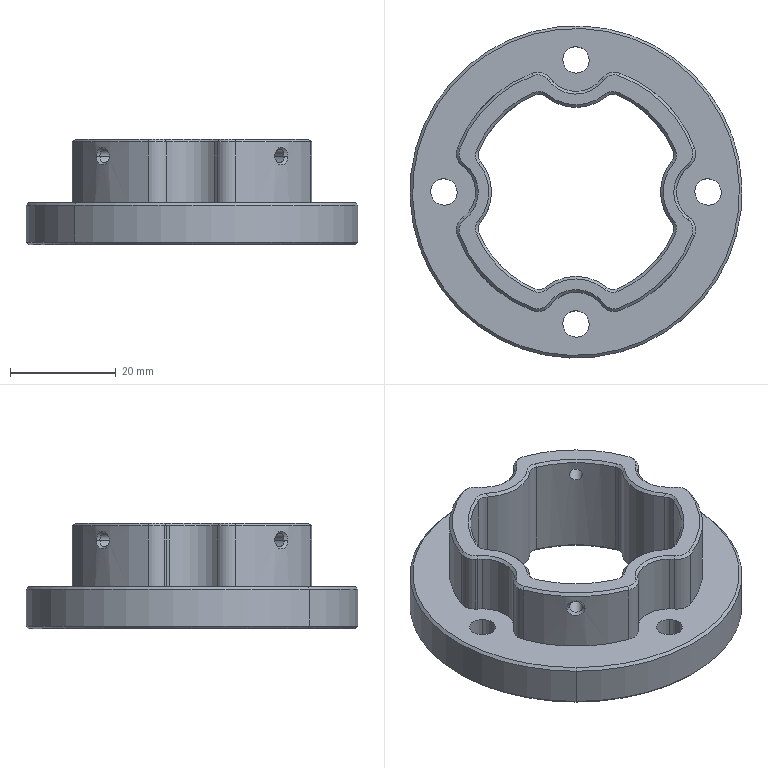NC program | NX | posted with a generic post | part box 62.9 x 62.9 x 20 mm
Lines 19 to 903 of 7695:
(ADAPTIVE_MILLING , TOOL : D10)
N36 T15 M6
N38 G54
N40 G17 G0 G90 X-44.154 Y6.39 S9500 M3
N42 G43 Z30. H15
N44 Z-8.9
N46 G94 G1 Z-11.9 F1000.
N48 X-43.177 Y6.446 F3000.
N50 X-42.201 Y6.527
N52 G3 X-41.498 Y7.102 R1.025
N54 X-40.854 Y10.262 R9.424
N56 X-40.658 Y21.758 R185.073
N58 G2 X-40.625 Y34.257 R639.071
N60 X-37.724 Y38.491 R6.067
N62 X-32.153 Y40.276 R13.146
N64 X-22.865 Y40.627 R85.364
N66 G1 X-21.065 Y40.633
N68 X-18.265 Y40.637
N70 X-12.065 Y40.639
N72 X33.735
N74 X33.835 Y40.637
N76 X33.935 Y40.634
N78 G2 X38.31 Y37.975 R5.843
N80 X40.247 Y32.358 R12.556
N82 X40.625 Y23.371 R77.114
N84 G1 X40.631 Y21.771
N86 X40.635 Y19.571
N88 X40.638 Y15.471
N90 X40.639 Y-15.229
N92 Y-33.729
N94 X40.638 Y-33.829
N96 G2 X37.978 Y-38.306 R5.815
N98 X32.461 Y-40.233 R12.425
N100 X24.476 Y-40.617 R66.82
N102 G1 X23.276 Y-40.625
N104 X21.676 Y-40.631
N106 X19.376 Y-40.636
N108 X15.076 Y-40.638
N110 X-33.724 Y-40.639
N112 X-33.824 Y-40.638
N114 G2 X-38.303 Y-37.982 R5.813
N116 X-40.22 Y-32.565 R12.366
N118 X-40.617 Y-24.481 R65.384
N120 G1 X-40.625 Y-23.381
N122 X-40.631 Y-21.781
N124 X-40.636 Y-19.481
N126 X-40.638 Y-15.281
N128 X-40.639 Y3.719
N130 X-40.637 Y3.919
N132 G2 X-40.169 Y9.298 R115.764
N134 G3 X-39.871 Y21.891 R175.546
N136 G1 X-39.867 Y24.891
N138 X-39.865 Y30.991
N140 X-39.863 Y31.091
N142 X-39.861 Y31.191
N144 X-39.853 Y31.391
N146 X-39.847 Y31.491
N148 X-39.84 Y31.59
N150 G2 X-36.002 Y37.476 R7.669
N152 X-29.749 Y39.423 R15.539
N154 X-19.762 Y39.816 R92.027
N156 G1 X-18.062 Y39.822
N158 X-15.662 Y39.827
N160 X-11.462 Y39.829
N162 X11.738 Y39.83
N164 X30.938
N166 X31.138 Y39.829
N168 G2 X37.449 Y36.019 R7.595
N170 X39.403 Y29.871 R15.313
N172 X39.808 Y20.986 R79.126
N174 G1 X39.816 Y19.686
N176 X39.822 Y17.986
N178 X39.827 Y15.486
N180 X39.829 Y11.186
N182 X39.83 Y-16.914
N184 Y-30.914
N186 G2 X36.123 Y-37.383 R7.547
N188 X29.795 Y-39.414 R15.249
N190 X20.609 Y-39.811 R83.586
N192 G1 X19.209 Y-39.818
N194 X17.309 Y-39.824
N196 X14.409 Y-39.828
N198 X8.509 Y-39.83
N200 X-30.991
N202 X-31.091
N204 G2 X-37.425 Y-36.057 R7.589
N206 X-39.413 Y-29.818 R15.258
N208 X-39.81 Y-20.632 R83.029
N210 G1 X-39.818 Y-19.132
N212 X-39.824 Y-17.232
N214 X-39.828 Y-14.332
N216 X-39.83 Y-8.332
N218 Y1.668
N220 X-39.827 Y2.068
N222 G2 X-39.346 Y9.852 R183.612
N224 G3 X-39.076 Y27.048 R323.967
N226 G2 X-38.811 Y31.028 R16.814
N228 X-33.821 Y36.948 R9.086
N230 X-26.878 Y38.692 R19.542
N232 X-15.986 Y39.011 R133.202
N234 G1 X-13.786 Y39.016
N236 X-10.386 Y39.02
N238 X-2.386 Y39.021
N240 X28.614
N242 X28.814 Y39.02
N244 X29.014 Y39.016
N246 G2 X36.75 Y34.168 R8.812
N248 X38.616 Y27.57 R18.024
N250 X39.001 Y18.082 R95.38
N252 G1 X39.009 Y16.582
N254 X39.015 Y14.582
N256 X39.019 Y11.682
N258 X39.021 Y5.982
N260 Y-28.618
N262 X39.02 Y-28.818
N264 G2 X34.163 Y-36.752 R8.824
N266 X27.365 Y-38.636 R18.17
N268 X16.675 Y-39.007 R112.972
N270 G1 X14.875 Y-39.014
N272 X12.276 Y-39.018
N274 X7.576 Y-39.021
N276 X-26.124 Y-39.022
N278 X-28.624 Y-39.021
N280 X-28.924 Y-39.018
N282 G2 X-36.708 Y-34.246 R8.797
N284 X-38.627 Y-27.459 R17.966
N286 X-39.008 Y-16.471 R114.033
N288 G1 X-39.014 Y-14.571
N290 X-39.019 Y-11.771
N292 X-39.021 Y-6.571
N294 Y0.029
N296 X-39.018 Y0.529
N298 X-39.012 Y1.029
N300 G2 X-38.485 Y11.415 R472.51
N302 G3 X-38.266 Y27.212 R522.18
N304 G2 X-32.726 Y35.942 R9.729
N306 X-25.911 Y37.789 R19.648
N308 X-14.624 Y38.197 R113.317
N310 G1 X-12.724 Y38.204
N312 X-10.124 Y38.209
N314 X-5.724 Y38.212
N316 X10.776 Y38.213
N318 X26.476
N320 X26.776 Y38.211
N322 G2 X36.02 Y32.533 R9.762
N324 X37.86 Y25.203 R20.771
N326 X38.204 Y12.812 R149.811
N328 G1 X38.209 Y10.212
N330 X38.212 Y5.812
N332 X38.213 Y-10.688
N334 Y-26.488
N336 X38.211 Y-26.788
N338 X38.207 Y-26.988
N340 G2 X32.609 Y-35.98 R9.723
N342 X25.686 Y-37.808 R19.975
N344 X14.497 Y-38.198 R118.542
N346 G1 X12.597 Y-38.204
N348 X9.997 Y-38.209
N350 X5.497 Y-38.212
N352 X-12.803 Y-38.213
N354 X-26.503
N356 X-26.803 Y-38.211
N358 G2 X-35.987 Y-32.599 R9.746
N360 X-37.832 Y-25.476 R20.283
N362 X-38.201 Y-13.686 R131.503
N364 X-38.158 Y1.813 R695.009
N366 G3 X-37.586 Y15.301 R684.53
N368 G2 X-37.441 Y26.099 R805.731
N370 X-31.332 Y35.151 R10.389
N372 X-24.004 Y37.007 R21.646
N374 X-13.314 Y37.384 R121.368
N376 G1 X-11.614 Y37.392
N378 X-9.314 Y37.398
N380 X-6.014 Y37.402
N382 X0.686 Y37.404
N384 X24.686
N386 X24.886 Y37.403
N388 G2 X30.856 Y36.034 R11.659
N390 X35.671 Y30.094 R11.361
N392 X37.144 Y22.363 R26.659
N394 X37.4 Y7.967 R242.401
N396 G1 X37.403 Y3.567
N398 X37.404 Y-11.633
N400 Y-24.633
N402 X37.403 Y-24.833
N404 X37.397 Y-25.232
N406 X37.393 Y-25.432
N408 G2 X34.427 Y-32.947 R10.423
N410 X27.757 Y-36.386 R13.873
N412 X19.32 Y-37.29 R43.09
N414 X2.72 Y-37.403 R760.11
N416 G1 X-18.28 Y-37.404
N418 X-24.68
N420 X-24.979 Y-37.402
N422 X-25.379 Y-37.395
N424 X-25.579 Y-37.39
N426 X-25.779 Y-37.382
N428 G2 X-35.059 Y-31.472 R10.331
N430 X-37.006 Y-23.965 R21.227
N432 X-37.39 Y-12.175 R132.868
N434 X-37.295 Y2.723 R384.936
N436 G3 X-36.678 Y24.012 R473.575
N438 G2 X-34.552 Y30.768 R11.574
N440 X-28.011 Y35.141 R12.771
N442 X-19.929 Y36.39 R32.975
N444 X-3.032 Y36.594 R394.511
N446 G1 X5.668 Y36.596
N448 X22.868
N450 X23.468 Y36.59
N452 X23.768 Y36.585
N454 X24.068 Y36.577
N456 G2 X31.057 Y34.264 R11.324
N458 X35.223 Y27.696 R13.034
N460 X36.406 Y19.501 R34.517
N462 X36.594 Y2.504 R426.496
N464 G1 X36.596 Y-7.396
N466 Y-22.896
N468 X36.59 Y-23.496
N470 X36.587 Y-23.696
N472 X36.576 Y-24.096
N474 G2 X34.118 Y-31.232 R11.22
N476 X27.475 Y-35.287 R13.274
N478 X19.371 Y-36.413 R35.677
N480 X5.273 Y-36.592 R366.726
N482 G1 X0.173 Y-36.595
N484 X-22.827 Y-36.596
N486 X-23.127 Y-36.595
N488 X-23.527 Y-36.589
N490 X-23.927 Y-36.581
N492 X-24.126 Y-36.574
N494 G2 X-31.332 Y-34.036 R11.175
N496 X-35.323 Y-27.351 R13.41
N498 X-36.427 Y-19.043 R36.843
N500 X-36.171 Y10.047 R355.609
N502 G3 X-35.886 Y22.644 R750.66
N504 G2 X-33.985 Y29.285 R12.572
N506 X-27.318 Y34.141 R12.741
N508 X-19.162 Y35.537 R31.275
N510 X-4.366 Y35.782 R280.79
N512 G1 X0.034 Y35.786
N514 X12.034 Y35.787
N516 X21.234
N518 X21.834 Y35.781
N520 X22.234 Y35.775
N522 X22.434 Y35.77
N524 G2 X28.859 Y34.17 R12.771
N526 X33.942 Y27.81 R12.264
N528 X35.481 Y19.886 R28.128
N530 X35.78 Y5.592 R220.124
N532 G1 X35.785 Y2.192
N534 X35.787 Y-4.408
N536 Y-21.308
N538 X35.785 Y-21.708
N540 X35.779 Y-22.108
N542 X35.77 Y-22.508
N544 G2 X34.026 Y-29.093 R12.572
N546 X27.456 Y-34.07 R12.532
N548 X19.411 Y-35.514 R29.843
N550 X4.516 Y-35.782 R258.634
N552 G1 X0.316 Y-35.786
N554 X-10.084 Y-35.787
N556 X-21.284
N558 X-21.884 Y-35.781
N560 X-22.184 Y-35.777
N562 X-22.584 Y-35.766
N564 G2 X-29.326 Y-33.879 R12.376
N566 X-34.163 Y-27.198 R12.759
N568 X-35.523 Y-19.338 R31.138
N570 X-35.778 Y-3.042 R287.727
N572 X-35.261 Y13.849 R960.15
N574 X-35.022 Y22.444 R183.444
N576 X-27.881 Y32.632 R11.828
N578 X-19.948 Y34.554 R24.698
N580 X-8.459 Y34.955 R134.916
N582 G1 X-6.959 Y34.963
N584 X-4.959 Y34.97
N586 X-2.059 Y34.974
N588 X2.841 Y34.978
N590 X19.641 Y34.979
N592 X20.141 Y34.976
N594 G2 X26.05 Y34.14 R17.215
N596 X32.764 Y27.517 R11.889
N598 X34.566 Y19.757 R25.348
N600 X34.961 Y7.367 R147.215
N602 G1 X34.969 Y5.267
N604 X34.974 Y2.467
N606 X34.977 Y-2.033
N608 X34.979 Y-14.333
N610 X34.978 Y-19.833
N612 X34.977 Y-20.133
N614 G2 X34.213 Y-25.854 R17.552
N616 X27.705 Y-32.677 R11.823
N618 X20.063 Y-34.535 R24.423
N620 X7.375 Y-34.961 R140.259
N622 G1 X5.275 Y-34.969
N624 X2.375 Y-34.974
N626 X-2.225 Y-34.977
N628 X-15.225 Y-34.979
N630 X-19.725 Y-34.978
N632 X-20.125 Y-34.976
N634 G2 X-26.036 Y-34.148 R17.243
N636 X-32.634 Y-27.807 R11.793
N638 X-34.564 Y-19.775 R24.739
N640 X-34.962 Y-7.185 R150.047
N642 X-34.53 Y11.708 R466.509
N644 X-34.245 Y21.103 R252.318
N646 X-30.784 Y29.092 R12.363
N648 X-23.638 Y32.911 R15.397
N650 X-14.321 Y34.016 R44.534
N652 X9.177 Y34.17 R850.322
N654 X20.776 Y34.105 R348.279
N656 X28.27 Y31.428 R12.545
N658 X32.61 Y24.608 R14.088
N660 X33.922 Y16.231 R35.311
N662 X34.166 Y0.035 R327.22
N664 G1 X34.169 Y-4.765
N666 X34.17 Y-18.265
N668 X34.168 Y-18.765
N670 X34.16 Y-19.265
N672 X34.152 Y-19.665
N674 G2 X32.838 Y-26.077 R15.03
N676 X26.124 Y-32.062 R12.55
N678 X18.039 Y-33.791 R27.574
N680 X6.048 Y-34.151 R158.399
N682 G1 X3.948 Y-34.159
N684 X1.548 Y-34.164
N686 X-2.552 Y-34.168
N688 X-11.652 Y-34.17
N690 X-18.252
N692 X-18.852 Y-34.165
N694 G2 X-24.867 Y-33.347 R18.267
N696 X-31.777 Y-26.78 R12.083
N698 X-33.717 Y-18.851 R24.92
N700 X-34.145 Y-7.064 R133.048
N702 X-33.746 Y11.531 R521.596
N704 X-33.439 Y20.124 R169.021
N706 X-29.523 Y28.531 R12.614
N708 X-22.072 Y32.204 R16.367
N710 X-12.741 Y33.216 R49.308
N712 X10.657 Y33.361 R912.675
N714 X20.055 Y33.258 R166.649
N716 X28.363 Y29.591 R12.423
N718 X32.101 Y22.397 R15.794
N720 X33.204 Y12.978 R46.108
N722 X33.36 Y-5.82 R649.081
N724 X33.308 Y-19.319 R520.164
N726 X31.273 Y-26.338 R13.629
N728 X24.439 Y-31.473 R13.459
N730 X16.112 Y-33.037 R31.178
N732 X2.618 Y-33.35 R213.351
N734 G1 X-0.082 Y-33.355
N736 X-4.082 Y-33.359
N738 X-12.682 Y-33.361
N740 X-16.882
N742 X-17.482 Y-33.356
N744 X-18.082 Y-33.347
N746 G2 X-24.266 Y-32.348 R17.235
N748 X-30.97 Y-25.68 R12.456
N750 X-32.914 Y-17.547 R25.856
N752 X-33.316 Y-2.758 R151.885
N754 X-33.089 Y6.739 R611.107
N756 X-32.703 Y18.432 R406.653
N758 X-30.307 Y25.748 R14.076
N760 X-23.14 Y30.775 R14.212
N762 X-14.591 Y32.25 R33.829
N764 X1.604 Y32.547 R280.622
N766 X18.003 Y32.502 R718.96
N768 X24.987 Y30.664 R14.521
N770 X30.579 Y23.584 R13.493
N772 X32.203 Y15.168 R30.977
N774 X32.543 Y0.375 R220.032
N776 X32.503 Y-18.025 R842.566
N778 X30.551 Y-25.177 R14.375
N780 X23.659 Y-30.551 R13.569
N782 X15.347 Y-32.19 R30.306
N784 X1.255 Y-32.541 R202.046
N786 G1 X-1.445 Y-32.547
N788 X-5.545 Y-32.551
N790 X-14.045 Y-32.553
N792 X-15.645 Y-32.552
N794 X-16.245 Y-32.549
N796 X-16.745 Y-32.541
N798 G2 X-22.949 Y-31.632 R18.901
N800 X-30.098 Y-24.75 R12.628
N802 X-32.106 Y-16.326 R26.295
N804 X-32.487 Y-1.637 R144.765
N806 X-31.935 Y17.154 R631.236
N808 X-29.939 Y24.1 R15.089
N810 X-22.755 Y29.729 R13.907
N812 X-14.342 Y31.371 R31.231
N814 X-1.149 Y31.727 R191.229
N816 X16.55 Y31.702 R884.582
N818 X23.33 Y30.205 R15.959
N820 X29.526 Y23.148 R13.281
N822 X31.338 Y14.673 R29.244
N824 X31.729 Y0.582 R186.623
N826 X31.695 Y-16.818 R780.638
N828 X30.036 Y-23.655 R15.347
N830 X22.995 Y-29.591 R13.469
N832 X14.707 Y-31.336 R29.368
N834 X0.916 Y-31.728 R180.86
N836 X-16.883 Y-31.691 R726.882
N838 X-23.799 Y-29.957 R15.111
N840 X-29.578 Y-23.029 R13.489
N842 X-31.362 Y-14.445 R29.894
N844 X-31.601 Y1.746 R164.804
N846 X-31.147 Y16.138 R407.692
N848 X-29.054 Y23.26 R15.315
N850 X-21.852 Y28.874 R14.108
N852 X-13.144 Y30.568 R31.918
N854 X1.648 Y30.924 R222.232
N856 X15.648 Y30.882 R578.884
N858 X22.596 Y29.251 R15.856
N860 X28.64 Y22.303 R13.463
N862 X30.501 Y13.839 R29.013
N864 X30.914 Y0.749 R163.434
N866 X30.886 Y-15.65 R709.93
N868 X29.252 Y-22.598 R15.884
N870 X22.118 Y-28.719 R13.567
N872 X13.639 Y-30.521 R29.782
N874 X0.949 Y-30.912 R168.52
N876 X-15.75 Y-30.881 R618.315
N878 X-22.599 Y-29.255 R15.737
N880 X-28.682 Y-22.213 R13.552
N882 X-30.503 Y-13.841 R29.011
N884 X-30.793 Y1.249 R143.854
N886 X-30.368 Y15.041 R354.424
N888 X-28.327 Y22.185 R15.914
N890 X-21.128 Y27.958 R14.207
N892 X-12.536 Y29.716 R31.047
N894 X1.055 Y30.107 R179.958
N896 X14.754 Y30.063 R430.554
N898 X21.784 Y28.352 R15.989
N900 X27.875 Y21.185 R13.8
N902 X29.691 Y12.708 R29.863
N904 X30.111 Y-1.881 R184.764
N906 X30.054 Y-14.98 R357.073
N908 X28.144 Y-22.155 R15.422
N910 X20.978 Y-27.963 R14.017
N912 X12.486 Y-29.713 R30.736
N914 X-1.705 Y-30.11 R189.354
N916 X-14.904 Y-30.057 R375.136
N918 X-21.914 Y-28.279 R15.627
N920 X-27.784 Y-21.42 R13.724
N922 X-29.7 Y-12.663 R29.361
N924 X-29.953 Y2.528 R147.815
N926 X-29.567 Y14.22 R242.398
N928 X-27.354 Y21.514 R15.754
N930 X-19.967 Y27.214 R14.541
N932 X-11.262 Y28.926 R32.658
N934 X2.23 Y29.298 R193.523
N936 X13.829 Y29.245 R301.238
N938 X20.857 Y27.52 R16.145
N940 X27.102 Y20.104 R14.055
N942 X28.88 Y11.618 R30.801
N944 X29.295 Y-1.672 R168.302
N946 X29.235 Y-14.071 R290.213
N948 X27.353 Y-21.155 R15.684
N950 X19.975 Y-27.155 R14.144
N952 X11.38 Y-28.905 R31.529
N954 X-2.01 Y-29.297 R182.206
N956 X-13.909 Y-29.24 R308.785
N958 X-21.014 Y-27.43 R15.897
N960 X-27.061 Y-20.217 R14.025
N962 X-28.911 Y-11.24 R30.857
N964 X-29.121 Y3.253 R150.199
N966 X-28.748 Y13.544 R166.987
N968 X-26.19 Y21.129 R15.346
N970 X-18.583 Y26.553 R15.107
N972 X-9.652 Y28.158 R35.45
N974 X6.242 Y28.499 R259.089
N976 X14.236 Y28.325 R86.731
N978 X22.699 Y24.672 R13.839
N980 X26.966 Y17.096 R16.45
N982 X28.278 Y7.505 R43.892
N984 X28.435 Y-12.791 R341.832
N986 X26.653 Y-20.008 R16.436
N988 X19.325 Y-26.214 R14.125
N990 X10.752 Y-28.054 R30.216
N992 X-3.538 Y-28.49 R180.341
N994 X-13.435 Y-28.393 R166.547
N996 X-20.986 Y-26.054 R15.058
N998 X-26.414 Y-18.814 R14.653
N1000 X-28.115 Y-9.905 R32.989
N1002 X-28.297 Y3.589 R145.776
N1004 X-27.939 Y12.78 R127.958
N1006 X-25.241 Y20.418 R15.291
N1008 X-17.759 Y25.696 R15.302
N1010 X-10.069 Y27.247 R35.598
N1012 X-7.887 Y27.73 R9.388
N1014 G3 X6.761 Y27.73 R374.985
N1016 G2 X14.247 Y27.388 R56.312
N1018 X25.007 Y19.273 R13.607
N1020 X27.115 Y10.973 R27.235
N1022 G3 X27.269 Y10.003 R6.674
N1024 G2 X27.728 Y6.561 R9.435
N1026 G3 X27.72 Y-8.786 R480.733
N1028 G2 X27.146 Y-15.549 R33.036
N1030 X19.617 Y-24.848 R13.474
N1032 X11.35 Y-27.07 R26.12
N1034 G3 X8.415 Y-27.667 R14.624
N1036 G2 X3.962 Y-27.67 R54.526
N1038 X-10.26 Y-27.687 R749.013
N1040 X-16.873 Y-26.777 R22.801
N1042 X-25.011 Y-19.276 R13.604
N1044 X-27.136 Y-10.674 R27.209
N1046 G3 X-27.516 Y-9.201 R6.554
N1048 G2 X-27.689 Y-6.116 R10.038
N1050 G3 X-27.474 Y5.18 R696.749
N1052 G2 X-27.569 Y9.108 R9.238
N1054 X-26.546 Y15.215 R37.091
N1056 X-18.57 Y24.184 R14.105
N1058 X-13.236 Y25.851 R25.594
N1060 G1 X-10.069 Y27.247
N1062 G2 X-7.887 Y27.73 R8.71
N1064 G1 X-6.219 Y27.687
N1066 G3 X-0.369 Y26.961 R22.412
N1068 G1 X0.23 Y26.947
N1070 X0.93 Y26.935
N1072 X1.73 Y26.926
N1074 X2.73 Y26.918
N1076 X3.53 Y26.915
N1078 X3.63 Y26.922
N1080 X3.729 Y26.937
N1082 G2 X6.547 Y27.72 R9.23
N1084 G3 X6.343 Y29.901 R1.1
N1086 G1 X4.344 Y29.834 Z-11.8
N1088 X-3.496 Y29.566
N1090 X-4.145 Y29.549 Z-11.833
N1092 X-4.793 Y29.508 Z-11.865
N1094 G3 X-5.394 Y29.171 Z-11.9 R1.144
N1096 X-4.845 Y27.361 R1.102
N1098 G2 X-3.497 Y26.854 R12.893
N1100 G3 X2.449 Y26.247 R20.794
N1102 X3.37 Y26.765 R3.244
N1104 G1 X3.923 Y26.998
N1106 G3 X4.401 Y28.637 R1.103
N1108 X3.408 Y29.113 Z-11.843 R1.131
N1110 G1 X2.559 Y29.117 Z-11.8
N1112 X-2.62 Y29.147
N1114 X-3.18 Y29.154 Z-11.828
N1116 X-3.741 Y29.139 Z-11.856
N1118 G3 X-4.469 Y28.689 Z-11.9 R1.128
N1120 X-4.058 Y27.066 R1.103
N1122 X1.627 Y25.68 R10.558
N1124 X2.819 Y26.392 R3.71
N1126 X2.224 Y28.391 R1.101
N1128 G1 X-2.324 Y28.549
N1130 G3 X-2.952 Y26.521 R1.101
N1132 X1.156 Y25.238 R5.804
N1134 X1.945 Y25.777 R1.631
N1136 G1 X2.026 Y25.834
N1138 G3 X1.507 Y27.828 R1.101
N1140 G1 X-1.745 Y28.165
N1142 G3 X-2.544 Y26.211 R1.101
N1144 X0.386 Y24.853 R4.842
N1146 X1.698 Y25.526 R1.473
N1148 X1.016 Y27.362 R1.101
N1150 G1 X-1.027 Y27.602
N1152 G3 X-1.841 Y25.65 R1.101
N1154 X-0.598 Y24.766 R4.738
N1156 X1.025 Y24.814 R1.654
N1158 G1 X1.102 Y24.878
N1160 X1.373 Y25.172
N1162 G3 X0.715 Y27.006 R1.101
N1164 G1 X0.011 Y27.11
N1166 X-0.697 Y27.189
N1168 G3 X-1.505 Y25.37 R1.101
N1170 X0.344 Y24.385 R2.116
N1172 X1.11 Y24.886 R1.337
N1174 X0.436 Y26.722 R1.101
N1176 G1 X0.026 Y26.774
N1178 X-0.386 Y26.81
N1180 G3 X-1.179 Y24.992 R1.101
N1182 X0.144 Y24.233 R1.554
N1184 X0.932 Y24.692 R1.248
N1186 X-1.144 Y25.935 R-1.233
N1188 X-0.917 Y24.689 R1.261
N1190 X0.712 Y24.469 R1.083
N1192 G1 X0.797 Y24.545
N1194 X1.86 Y25.703
N1196 X1.945 Y25.777
N1198 G2 X4.973 Y27.427 R9.279
N1200 G1 X6.661 Y27.733
N1202 X6.761 Y27.73
N1204 G2 X9.871 Y27.307 R9.014
N1206 X14.975 Y26.325 R72.636
N1208 X24.226 Y18.271 R13.984
N1210 X25.819 Y13.273 R29.214
N1212 X27.242 Y10.083 R41.896
N1214 G3 X28.775 Y9.69 R1.003
N1216 X29.176 Y10.531 Z-11.852 R1.137
N1218 G1 X29.316 Y11.559 Z-11.8
N1220 X29.455 Y12.566
N1222 X29.579 Y13.575
N1224 X29.553 Y13.781
N1226 X29.492 Y13.98
N1228 X27.962 Y17.399
N1230 X26.396 Y20.802
N1232 G3 X25.029 Y22.866 R9.239
N1234 G1 X23.629 Y24.461
N1236 X22.211 Y26.038
N1238 G3 X19.802 Y27.776 R9.636
N1240 G1 X19.128 Y28.101
N1242 X18.44 Y28.392
N1244 X12.857 Y30.533
N1246 G3 X12.056 Y30.495 R1.026
N1248 G1 X10.524 Y29.737
N1250 X9.923 Y29.445 Z-11.833
N1252 X9.333 Y29.131 Z-11.867
N1254 G3 X8.958 Y28.599 Z-11.9 R1.04
N1256 X9.676 Y27.351 R1.004
N1258 G2 X11.558 Y26.623 R15.109
N1260 X16.247 Y24.898 R43.642
N1262 X23.698 Y16.731 R15.105
N1264 X25.823 Y13.266 R25.695
N1266 G3 X27.669 Y13.539 R1.001
N1268 X27.633 Y14.204 Z-11.867 R1.689
N1270 G1 X27.414 Y15.515 Z-11.8
N1272 X27.096 Y17.375
N1274 X26.988 Y17.613
N1276 X25.636 Y19.785
N1278 X24.27 Y21.947
N1280 G3 X22.073 Y24.696 R21.386
N1282 X19.539 Y26.601 R10.917
N1284 G1 X15.082 Y29.016
N1286 G3 X14.457 Y29.126 R1.042
N1288 G1 X12.673 Y28.859
N1290 X11.979 Y28.758 Z-11.835
N1292 X11.287 Y28.641 Z-11.87
N1294 G3 X10.801 Y28.311 Z-11.9 R1.049
N1296 X11.184 Y26.766 R1.003
N1298 G1 X12.908 Y26.023
N1300 X12.959 Y25.998
N1302 G2 X17.491 Y23.171 R33.094
N1304 X20.588 Y20.493 R35.872
N1306 G1 X22.637 Y18.204
N1308 X22.672 Y18.16
N1310 X23.722 Y16.698
N1312 G3 X25.38 Y18.13 R-1.1
N1314 G1 X17.103 Y26.126
N1316 G3 X15.696 Y24.443 R-1.1
N1318 G1 X17.806 Y22.923
N1320 G2 X20.588 Y20.493 R35.704
N1322 X24.494 Y15.616 R33.992
N1324 G1 X26.031 Y12.891
N1326 X27.269 Y10.003
N1328 G2 X27.733 Y6.661 R9.461
N1330 G3 X27.063 Y2.403 R37.637
N1332 X26.934 Y-3.694 R104.126
N1334 G1 X27.346 Y-4.71
N1336 X27.687 Y-6.21
N1338 X27.7 Y-6.316
N1340 G3 X29.854 Y-6.465 R1.1
N1342 G1 X29.892 Y-6.111 Z-11.882
N1344 X29.88 Y-5.756 Z-11.864
N1346 X29.843 Y-4.469 Z-11.8
N1348 X29.609 Y3.686
N1350 X29.595 Y4.27 Z-11.829
N1352 X29.563 Y4.854 Z-11.859
N1354 G3 X29.135 Y5.542 Z-11.9 R1.13
N1356 X27.427 Y4.973 R1.102
N1358 X26.334 Y0.319 R12.438
N1360 X26.258 Y-2.476 R18.046
N1362 X26.676 Y-3.209 R2.933
N1364 G1 X27.007 Y-3.937
N1366 G3 X28.622 Y-4.395 R1.103
N1368 X29.108 Y-3.299 Z-11.837 R1.19
N1370 G1 X29.11 Y-2.559 Z-11.8
N1372 X29.119 Y2.501
N1374 X29.123 Y3.09 Z-11.829
N1376 X29.109 Y3.679 Z-11.859
N1378 G3 X28.71 Y4.375 Z-11.9 R1.13
N1380 X27.007 Y3.944 R1.103
N1382 G1 X26.765 Y3.37
N1384 X26.711 Y3.272
N1386 X26.656 Y3.188
N1388 X26.604 Y3.103
N1390 X26.556 Y3.015
N1392 X26.509 Y2.927
N1394 X26.465 Y2.837
N1396 X26.423 Y2.746
N1398 X26.383 Y2.655
N1400 X26.344 Y2.563
N1402 X26.308 Y2.47
N1404 X26.273 Y2.376
N1406 G3 X25.688 Y-1.655 R10.536
N1408 X26.42 Y-2.84 R3.647
N1410 X28.407 Y-2.26 R1.101
N1412 G1 X28.708 Y2.57
N1414 G3 X26.711 Y3.272 R1.101
N1416 X25.225 Y-1.072 R6.432
N1418 X25.716 Y-1.874 R1.396
N1420 G1 X25.833 Y-2.035
N1422 G3 X27.817 Y-1.494 R1.101
N1424 G1 X28.13 Y1.714
N1426 G3 X26.136 Y2.454 R1.101
N1428 X25.046 Y0.634 R6.657
N1430 X24.997 Y-1.123 R2.397
N1432 X25.543 Y-1.702 R3.429
N1434 X27.378 Y-0.981 R1.101
N1436 G1 X27.543 Y0.957
N1438 G3 X25.703 Y1.86 R1.101
N1440 X24.633 Y-0.677 R2.61
N1442 X25.181 Y-1.374 R1.696
N1444 X27.012 Y-0.695 R1.101
N1446 G1 X27.108 Y0.028
N1448 X27.178 Y0.754
N1450 G3 X25.335 Y1.522 R1.101
N1452 X24.384 Y-0.35 R2.169
N1454 X24.888 Y-1.107 R1.341
N1456 X26.719 Y-0.429 R1.101
N1458 G1 X26.772 Y-0.008
N1460 X26.81 Y0.416
N1462 G3 X24.966 Y1.184 R1.101
N1464 X24.231 Y-0.154 R1.583
N1466 X24.696 Y-0.933 R1.257
N1468 X26.41 Y0.691 R1.185
N1470 X24.598 Y0.846 R1.238
N1472 X24.468 Y-0.709 R1.071
N1474 G1 X24.548 Y-0.799
N1476 X25.139 Y-1.328
N1478 X25.716 Y-1.874
N1480 X26.205 Y-2.534
N1482 X26.676 Y-3.209
N1484 X27.021 Y-3.955
N1486 X27.346 Y-4.71
N1488 X27.534 Y-5.511
N1490 X27.7 Y-6.316
N1492 X27.73 Y-7.886
N1494 G2 X27.186 Y-10.617 R28.474
N1496 X25.952 Y-16.173 R31.711
N1498 X18.043 Y-24.332 R14.053
N1500 X13.278 Y-25.816 R28.776
N1502 X10.083 Y-27.242 R42.262
N1504 G3 X9.69 Y-28.775 R1.003
N1506 X10.531 Y-29.176 Z-11.852 R1.137
N1508 G1 X11.559 Y-29.316 Z-11.8
N1510 X12.566 Y-29.455
N1512 X13.575 Y-29.579
N1514 X13.781 Y-29.553
N1516 X13.98 Y-29.492
N1518 X17.399 Y-27.962
N1520 X20.802 Y-26.396
N1522 G3 X22.877 Y-25.04 R9.685
N1524 G1 X25.709 Y-22.592
N1526 G3 X26.779 Y-21.465 R7.385
N1528 X28.398 Y-18.453 R14.727
N1530 G1 X30.655 Y-12.532
N1532 G3 X30.611 Y-11.721 R1.025
N1534 G1 X29.843 Y-10.217
N1536 X29.547 Y-9.626 Z-11.833
N1538 X29.23 Y-9.047 Z-11.866
N1540 G3 X28.677 Y-8.677 Z-11.9 R1.039
N1542 X27.473 Y-9.35 R1.005
N1544 G2 X26.562 Y-11.733 R29.9
N1546 X24.546 Y-16.948 R31.162
N1548 X16.767 Y-23.681 R15.085
N1550 X13.196 Y-25.863 R27.963
N1552 G3 X13.468 Y-27.709 R1.001
N1554 X14.133 Y-27.673 Z-11.866 R1.684
N1556 G1 X15.443 Y-27.455 Z-11.8
N1558 X17.305 Y-27.136
N1560 X17.542 Y-27.028
N1562 X19.715 Y-25.677
N1564 X21.877 Y-24.31
N1566 G3 X24.626 Y-22.114 R21.423
N1568 X26.541 Y-19.584 R11.112
N1570 G1 X29.022 Y-15.068
N1572 G3 X29.135 Y-14.438 R1.042
N1574 G1 X28.867 Y-12.661
N1576 X28.765 Y-11.966 Z-11.835
N1578 X28.646 Y-11.273 Z-11.87
N1580 G3 X28.318 Y-10.788 Z-11.9 R1.049
N1582 X26.772 Y-11.171 R1.003
N1584 G1 X26.027 Y-12.9
N1586 X26.002 Y-12.95
N1588 G2 X22.619 Y-18.227 R33.78
N1590 X18.182 Y-22.654 R33.779
N1592 G1 X16.64 Y-23.763
N1594 G3 X18.072 Y-25.421 R-1.1
N1596 G1 X26.137 Y-17.087
N1598 G3 X24.453 Y-15.68 R-1.1
N1600 G1 X22.935 Y-17.791
N1602 G2 X20.52 Y-20.56 R36.055
N1604 X15.632 Y-24.484 R34.001
N1606 G1 X12.9 Y-26.027
N1608 X10.003 Y-27.269
N1610 G2 X6.661 Y-27.733 R9.461
N1612 G3 X2.403 Y-27.063 R37.552
N1614 X-3.792 Y-26.953 R54.75
N1616 G1 X-3.87 Y-26.976
N1618 X-4.866 Y-27.395
N1620 X-4.973 Y-27.427
N1622 X-6.547 Y-27.72
N1624 G3 X-6.394 Y-29.9 R1.1
N1626 G1 X-4.394 Y-29.845 Z-11.8
N1628 X3.682 Y-29.61
N1630 X4.268 Y-29.595 Z-11.829
N1632 X4.854 Y-29.564 Z-11.859
N1634 G3 X5.54 Y-29.138 Z-11.9 R1.13
N1636 X4.973 Y-27.427 R1.102
N1638 X0.119 Y-26.318 R12.805
N1640 X-2.476 Y-26.255 R19.49
N1642 X-3.37 Y-26.765 R3.444
N1644 G1 X-3.923 Y-26.998
N1646 G3 X-4.396 Y-28.645 R1.103
N1648 X-3.403 Y-29.112 Z-11.843 R1.132
N1650 G1 X-2.55 Y-29.113 Z-11.8
N1652 X2.502 Y-29.12
N1654 X3.091 Y-29.123 Z-11.829
N1656 X3.68 Y-29.109 Z-11.859
N1658 G3 X4.376 Y-28.709 Z-11.9 R1.13
N1660 X3.944 Y-27.007 R1.103
N1662 G1 X3.37 Y-26.765
N1664 X3.272 Y-26.711
N1666 X3.189 Y-26.656
N1668 X3.103 Y-26.604
N1670 X3.016 Y-26.555
N1672 X2.927 Y-26.509
N1674 X2.838 Y-26.465
N1676 X2.747 Y-26.422
N1678 X2.655 Y-26.382
N1680 X2.563 Y-26.344
N1682 X2.47 Y-26.307
N1684 X2.376 Y-26.273
N1686 G3 X-1.655 Y-25.688 R10.535
N1688 X-2.834 Y-26.403 R3.948
N1690 X-2.271 Y-28.4 R1.101
N1692 G1 X2.569 Y-28.708
N1694 G3 X3.272 Y-26.711 R1.101
N1696 X-1.072 Y-25.225 R6.422
N1698 X-1.945 Y-25.777 R1.515
N1700 G1 X-2.026 Y-25.834
N1702 G3 X-1.496 Y-27.829 R1.101
N1704 G1 X1.719 Y-28.13
N1706 G3 X2.454 Y-26.136 R1.101
N1708 X0.634 Y-25.046 R6.676
N1710 X-1.124 Y-24.994 R2.428
N1712 X-1.706 Y-25.535 R3.354
N1714 X-0.991 Y-27.375 R1.101
N1716 G1 X0.956 Y-27.543
N1718 G3 X1.86 Y-25.703 R1.101
N1720 X-0.677 Y-24.629 R2.619
N1722 X-1.375 Y-25.175 R1.706
N1724 X-0.702 Y-27.01 R1.101
N1726 G1 X0.025 Y-27.107
N1728 X0.754 Y-27.178
N1730 G3 X1.522 Y-25.335 R1.101
N1732 X-0.35 Y-24.382 R2.172
N1734 X-1.172 Y-24.954 R1.482
N1736 X-0.381 Y-26.798 R1.101
N1738 G1 X0.072 Y-26.806
N1740 X0.525 Y-26.8
N1742 G3 X1.184 Y-24.966 R1.101
N1744 X-0.154 Y-24.23 R1.584
N1746 X-0.932 Y-24.692 R1.262
N1748 X0.689 Y-26.415 R1.187
N1750 X0.846 Y-24.598 R1.241
N1752 X-0.712 Y-24.469 R1.072
N1754 G1 X-0.797 Y-24.545
N1756 X-1.86 Y-25.703
N1758 X-1.945 Y-25.777
N1760 G2 X-4.973 Y-27.427 R9.279
N1762 G1 X-6.661 Y-27.733
N1764 X-6.761 Y-27.73
N1766 G2 X-9.676 Y-27.351 R8.469
N1768 X-14.685 Y-26.403 R121.65
N1770 X-24.35 Y-17.999 R14.062
N1772 X-25.814 Y-13.283 R30.181
N1774 X-27.247 Y-10.069 R41.917
N1776 G3 X-28.78 Y-9.676 R1.003
N1778 X-29.182 Y-10.518 Z-11.852 R1.137
N1780 G1 X-29.321 Y-11.546 Z-11.8
N1782 X-29.461 Y-12.553
N1784 X-29.585 Y-13.561
N1786 X-29.559 Y-13.768
N1788 X-29.497 Y-13.966
N1790 X-27.967 Y-17.386
N1792 X-26.401 Y-20.789
N1794 G3 X-25.046 Y-22.863 R9.685
N1796 G1 X-22.598 Y-25.696
N1798 G3 X-21.471 Y-26.765 R7.332